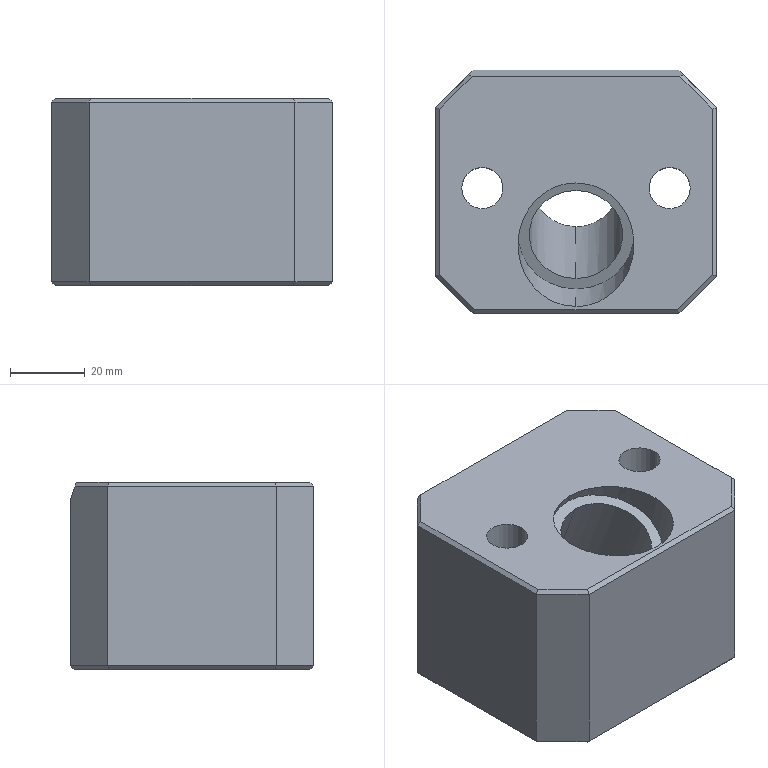Part | Creo | 3 solids | 45 faces | box 75 x 65 x 50 mm | volume 192089 mm3 | plane 29 | cylinder 16 | commonest cylinder face diameters 11 x4 18 x4 11.98 x2 12 x2 25 x2 31 x2
STEP:
#1=CARTESIAN_POINT('',(30.502,321.495,1.));
#2=VERTEX_POINT('',#1);
#3=CARTESIAN_POINT('',(19.502,321.495,1.));
#4=VERTEX_POINT('',#3);
#5=CARTESIAN_POINT('',(25.002,321.495,1.));
#6=DIRECTION('',(0.,0.,1.));
#7=DIRECTION('',(1.,0.,0.));
#8=AXIS2_PLACEMENT_3D('',#5,#6,#7);
#9=CIRCLE('',#8,5.5);
#10=EDGE_CURVE('',#2,#4,#9,.T.);
#11=ORIENTED_EDGE('',*,*,#10,.T.);
#12=CARTESIAN_POINT('',(19.502,321.495,40.));
#13=VERTEX_POINT('',#12);
#14=CARTESIAN_POINT('',(19.502,321.495,1.));
#15=DIRECTION('',(0.,0.,1.));
#16=VECTOR('',#15,39.);
#17=LINE('',#14,#16);
#18=EDGE_CURVE('',#4,#13,#17,.T.);
#19=ORIENTED_EDGE('',*,*,#18,.T.);
#20=CARTESIAN_POINT('',(30.502,321.495,40.));
#21=VERTEX_POINT('',#20);
#22=CARTESIAN_POINT('',(25.002,321.495,40.));
#23=DIRECTION('',(0.,0.,-1.));
#24=DIRECTION('',(-1.,0.,0.));
#25=AXIS2_PLACEMENT_3D('',#22,#23,#24);
#26=CIRCLE('',#25,5.5);
#27=EDGE_CURVE('',#13,#21,#26,.T.);
#28=ORIENTED_EDGE('',*,*,#27,.T.);
#29=CARTESIAN_POINT('',(30.502,321.495,1.));
#30=DIRECTION('',(0.,0.,1.));
#31=VECTOR('',#30,39.);
#32=LINE('',#29,#31);
#33=EDGE_CURVE('',#2,#21,#32,.T.);
#34=ORIENTED_EDGE('',*,*,#33,.F.);
#35=EDGE_LOOP('',(#11,#19,#28,#34));
#36=FACE_OUTER_BOUND('',#35,.F.);
#37=CARTESIAN_POINT('',(25.002,321.495,-10.));
#38=DIRECTION('',(0.,0.,1.));
#39=DIRECTION('',(-1.,0.,0.));
#40=AXIS2_PLACEMENT_3D('',#37,#38,#39);
#41=CYLINDRICAL_SURFACE('',#40,5.5);
#42=ADVANCED_FACE('',(#36),#41,.F.);
#43=CARTESIAN_POINT('',(16.002,321.495,1.));
#44=VERTEX_POINT('',#43);
#45=CARTESIAN_POINT('',(34.002,321.495,1.));
#46=VERTEX_POINT('',#45);
#47=CARTESIAN_POINT('',(25.002,321.495,1.));
#48=DIRECTION('',(0.,0.,-1.));
#49=DIRECTION('',(-1.,0.,0.));
#50=AXIS2_PLACEMENT_3D('',#47,#48,#49);
#51=CIRCLE('',#50,9.);
#52=EDGE_CURVE('',#44,#46,#51,.T.);
#53=ORIENTED_EDGE('',*,*,#52,.F.);
#54=CARTESIAN_POINT('',(25.002,321.495,1.));
#55=DIRECTION('',(0.,0.,-1.));
#56=DIRECTION('',(1.,0.,0.));
#57=AXIS2_PLACEMENT_3D('',#54,#55,#56);
#58=CIRCLE('',#57,9.);
#59=EDGE_CURVE('',#46,#44,#58,.T.);
#60=ORIENTED_EDGE('',*,*,#59,.F.);
#61=EDGE_LOOP('',(#53,#60));
#62=FACE_OUTER_BOUND('',#61,.F.);
#63=CARTESIAN_POINT('',(25.002,321.495,1.));
#64=DIRECTION('',(0.,0.,1.));
#65=DIRECTION('',(-1.,0.,0.));
#66=AXIS2_PLACEMENT_3D('',#63,#64,#65);
#67=CIRCLE('',#66,5.5);
#68=EDGE_CURVE('',#4,#2,#67,.T.);
#69=ORIENTED_EDGE('',*,*,#68,.F.);
#70=ORIENTED_EDGE('',*,*,#10,.F.);
#71=EDGE_LOOP('',(#69,#70));
#72=FACE_BOUND('',#71,.F.);
#73=CARTESIAN_POINT('',(25.002,321.495,1.));
#74=DIRECTION('',(0.,0.,1.));
#75=DIRECTION('',(-1.,0.,0.));
#76=AXIS2_PLACEMENT_3D('',#73,#74,#75);
#77=PLANE('',#76);
#78=ADVANCED_FACE('',(#62,#72),#77,.F.);
#79=ORIENTED_EDGE('',*,*,#52,.T.);
#80=CARTESIAN_POINT('',(34.002,321.495,-10.));
#81=VERTEX_POINT('',#80);
#82=CARTESIAN_POINT('',(34.002,321.495,-10.));
#83=DIRECTION('',(0.,0.,1.));
#84=VECTOR('',#83,11.);
#85=LINE('',#82,#84);
#86=EDGE_CURVE('',#81,#46,#85,.T.);
#87=ORIENTED_EDGE('',*,*,#86,.F.);
#88=CARTESIAN_POINT('',(16.002,321.495,-10.));
#89=VERTEX_POINT('',#88);
#90=CARTESIAN_POINT('',(25.002,321.495,-10.));
#91=DIRECTION('',(0.,0.,1.));
#92=DIRECTION('',(1.,0.,0.));
#93=AXIS2_PLACEMENT_3D('',#90,#91,#92);
#94=CIRCLE('',#93,9.);
#95=EDGE_CURVE('',#81,#89,#94,.T.);
#96=ORIENTED_EDGE('',*,*,#95,.T.);
#97=CARTESIAN_POINT('',(16.002,321.495,-10.));
#98=DIRECTION('',(0.,0.,1.));
#99=VECTOR('',#98,11.);
#100=LINE('',#97,#99);
#101=EDGE_CURVE('',#89,#44,#100,.T.);
#102=ORIENTED_EDGE('',*,*,#101,.T.);
#103=EDGE_LOOP('',(#79,#87,#96,#102));
#104=FACE_OUTER_BOUND('',#103,.F.);
#105=CARTESIAN_POINT('',(25.002,321.495,-10.));
#106=DIRECTION('',(0.,0.,1.));
#107=DIRECTION('',(-1.,0.,0.));
#108=AXIS2_PLACEMENT_3D('',#105,#106,#107);
#109=CYLINDRICAL_SURFACE('',#108,9.);
#110=ADVANCED_FACE('',(#104),#109,.F.);
#111=ORIENTED_EDGE('',*,*,#59,.T.);
#112=ORIENTED_EDGE('',*,*,#101,.F.);
#113=CARTESIAN_POINT('',(25.002,321.495,-10.));
#114=DIRECTION('',(0.,0.,1.));
#115=DIRECTION('',(-1.,0.,0.));
#116=AXIS2_PLACEMENT_3D('',#113,#114,#115);
#117=CIRCLE('',#116,9.);
#118=EDGE_CURVE('',#89,#81,#117,.T.);
#119=ORIENTED_EDGE('',*,*,#118,.T.);
#120=ORIENTED_EDGE('',*,*,#86,.T.);
#121=EDGE_LOOP('',(#111,#112,#119,#120));
#122=FACE_OUTER_BOUND('',#121,.F.);
#123=CARTESIAN_POINT('',(25.002,321.495,-10.));
#124=DIRECTION('',(0.,0.,1.));
#125=DIRECTION('',(-1.,0.,0.));
#126=AXIS2_PLACEMENT_3D('',#123,#124,#125);
#127=CYLINDRICAL_SURFACE('',#126,9.);
#128=ADVANCED_FACE('',(#122),#127,.F.);
#129=CARTESIAN_POINT('',(36.502,298.41,-10.));
#130=VERTEX_POINT('',#129);
#131=CARTESIAN_POINT('',(27.087,288.995,-10.));
#132=VERTEX_POINT('',#131);
#133=CARTESIAN_POINT('',(36.502,298.41,-10.));
#134=DIRECTION('',(-0.7071,-0.7071,0.));
#135=VECTOR('',#134,13.314);
#136=LINE('',#133,#135);
#137=EDGE_CURVE('',#130,#132,#136,.T.);
#138=ORIENTED_EDGE('',*,*,#137,.F.);
#139=CARTESIAN_POINT('',(36.502,342.581,-10.));
#140=VERTEX_POINT('',#139);
#141=CARTESIAN_POINT('',(36.502,298.41,-10.));
#142=DIRECTION('',(0.,1.,0.));
#143=VECTOR('',#142,44.172);
#144=LINE('',#141,#143);
#145=EDGE_CURVE('',#130,#140,#144,.T.);
#146=ORIENTED_EDGE('',*,*,#145,.T.);
#147=CARTESIAN_POINT('',(27.087,351.995,-10.));
#148=VERTEX_POINT('',#147);
#149=CARTESIAN_POINT('',(27.087,351.995,-10.));
#150=DIRECTION('',(0.7071,-0.7071,0.));
#151=VECTOR('',#150,13.314);
#152=LINE('',#149,#151);
#153=EDGE_CURVE('',#148,#140,#152,.T.);
#154=ORIENTED_EDGE('',*,*,#153,.F.);
#155=CARTESIAN_POINT('',(-27.084,351.995,-10.));
#156=VERTEX_POINT('',#155);
#157=CARTESIAN_POINT('',(27.087,351.995,-10.));
#158=DIRECTION('',(-1.,0.,0.));
#159=VECTOR('',#158,54.172);
#160=LINE('',#157,#159);
#161=EDGE_CURVE('',#148,#156,#160,.T.);
#162=ORIENTED_EDGE('',*,*,#161,.T.);
#163=CARTESIAN_POINT('',(-36.498,342.581,-10.));
#164=VERTEX_POINT('',#163);
#165=CARTESIAN_POINT('',(-36.498,342.581,-10.));
#166=DIRECTION('',(0.7071,0.7071,0.));
#167=VECTOR('',#166,13.314);
#168=LINE('',#165,#167);
#169=EDGE_CURVE('',#164,#156,#168,.T.);
#170=ORIENTED_EDGE('',*,*,#169,.F.);
#171=CARTESIAN_POINT('',(-36.498,298.41,-10.));
#172=VERTEX_POINT('',#171);
#173=CARTESIAN_POINT('',(-36.498,342.581,-10.));
#174=DIRECTION('',(0.,-1.,0.));
#175=VECTOR('',#174,44.172);
#176=LINE('',#173,#175);
#177=EDGE_CURVE('',#164,#172,#176,.T.);
#178=ORIENTED_EDGE('',*,*,#177,.T.);
#179=CARTESIAN_POINT('',(-27.084,288.995,-10.));
#180=VERTEX_POINT('',#179);
#181=CARTESIAN_POINT('',(-27.084,288.995,-10.));
#182=DIRECTION('',(-0.7071,0.7071,0.));
#183=VECTOR('',#182,13.314);
#184=LINE('',#181,#183);
#185=EDGE_CURVE('',#180,#172,#184,.T.);
#186=ORIENTED_EDGE('',*,*,#185,.F.);
#187=CARTESIAN_POINT('',(-27.084,288.995,-10.));
#188=DIRECTION('',(1.,0.,0.));
#189=VECTOR('',#188,54.172);
#190=LINE('',#187,#189);
#191=EDGE_CURVE('',#180,#132,#190,.T.);
#192=ORIENTED_EDGE('',*,*,#191,.T.);
#193=EDGE_LOOP('',(#138,#146,#154,#162,#170,#178,#186,#192));
#194=FACE_OUTER_BOUND('',#193,.F.);
#195=ORIENTED_EDGE('',*,*,#118,.F.);
#196=ORIENTED_EDGE('',*,*,#95,.F.);
#197=EDGE_LOOP('',(#195,#196));
#198=FACE_BOUND('',#197,.F.);
#199=CARTESIAN_POINT('',(-33.998,321.495,-10.));
#200=VERTEX_POINT('',#199);
#201=CARTESIAN_POINT('',(-15.998,321.495,-10.));
#202=VERTEX_POINT('',#201);
#203=CARTESIAN_POINT('',(-24.998,321.495,-10.));
#204=DIRECTION('',(0.,0.,1.));
#205=DIRECTION('',(-1.,0.,0.));
#206=AXIS2_PLACEMENT_3D('',#203,#204,#205);
#207=CIRCLE('',#206,9.);
#208=EDGE_CURVE('',#200,#202,#207,.T.);
#209=ORIENTED_EDGE('',*,*,#208,.F.);
#210=CARTESIAN_POINT('',(-24.998,321.495,-10.));
#211=DIRECTION('',(0.,0.,1.));
#212=DIRECTION('',(1.,0.,0.));
#213=AXIS2_PLACEMENT_3D('',#210,#211,#212);
#214=CIRCLE('',#213,9.);
#215=EDGE_CURVE('',#202,#200,#214,.T.);
#216=ORIENTED_EDGE('',*,*,#215,.F.);
#217=EDGE_LOOP('',(#209,#216));
#218=FACE_BOUND('',#217,.F.);
#219=CARTESIAN_POINT('',(0.,311.266,-10.));
#220=VERTEX_POINT('',#219);
#221=CARTESIAN_POINT('',(0.,337.871,-10.));
#222=VERTEX_POINT('',#221);
#223=CARTESIAN_POINT('',(0.,311.266,-10.));
#224=CARTESIAN_POINT('',(-1.473,311.266,-10.));
#225=CARTESIAN_POINT('',(-4.657,311.834,-10.));
#226=CARTESIAN_POINT('',(-8.358,314.374,-10.));
#227=CARTESIAN_POINT('',(-10.541,317.247,-10.));
#228=CARTESIAN_POINT('',(-11.706,319.657,-10.));
#229=CARTESIAN_POINT('',(-12.259,321.74,-10.));
#230=CARTESIAN_POINT('',(-12.467,323.38,-10.));
#231=CARTESIAN_POINT('',(-12.516,324.569,-10.));
#232=CARTESIAN_POINT('',(-12.467,325.757,-10.));
#233=CARTESIAN_POINT('',(-12.259,327.397,-10.));
#234=CARTESIAN_POINT('',(-11.706,329.48,-10.));
#235=CARTESIAN_POINT('',(-10.541,331.89,-10.));
#236=CARTESIAN_POINT('',(-8.358,334.763,-10.));
#237=CARTESIAN_POINT('',(-4.657,337.303,-10.));
#238=CARTESIAN_POINT('',(-1.473,337.871,-10.));
#239=CARTESIAN_POINT('',(0.,337.871,-10.));
#240=B_SPLINE_CURVE_WITH_KNOTS('',3,(#223,#224,#225,#226,#227,#228,#229,#230,#231,#232,#233,#234,#235,#236,#237,#238,#239),.UNSPECIFIED.,.F.,.F.,(4,1,1,1,1,1,1,1,1,1,1,1,1,1,4),(0.,0.125,0.25,0.3125,0.375,0.4375,0.4688,0.5,0.5312,0.5625,0.625,0.6875,0.75,0.875,1.),.UNSPECIFIED.);
#241=EDGE_CURVE('',#220,#222,#240,.T.);
#242=ORIENTED_EDGE('',*,*,#241,.T.);
#243=CARTESIAN_POINT('',(0.,337.871,-10.));
#244=CARTESIAN_POINT('',(1.473,337.871,-10.));
#245=CARTESIAN_POINT('',(4.657,337.303,-10.));
#246=CARTESIAN_POINT('',(8.358,334.763,-10.));
#247=CARTESIAN_POINT('',(10.541,331.89,-10.));
#248=CARTESIAN_POINT('',(11.706,329.48,-10.));
#249=CARTESIAN_POINT('',(12.259,327.397,-10.));
#250=CARTESIAN_POINT('',(12.467,325.757,-10.));
#251=CARTESIAN_POINT('',(12.516,324.569,-10.));
#252=CARTESIAN_POINT('',(12.467,323.38,-10.));
#253=CARTESIAN_POINT('',(12.259,321.74,-10.));
#254=CARTESIAN_POINT('',(11.706,319.657,-10.));
#255=CARTESIAN_POINT('',(10.541,317.247,-10.));
#256=CARTESIAN_POINT('',(8.358,314.374,-10.));
#257=CARTESIAN_POINT('',(4.657,311.834,-10.));
#258=CARTESIAN_POINT('',(1.473,311.266,-10.));
#259=CARTESIAN_POINT('',(0.,311.266,-10.));
#260=B_SPLINE_CURVE_WITH_KNOTS('',3,(#243,#244,#245,#246,#247,#248,#249,#250,#251,#252,#253,#254,#255,#256,#257,#258,#259),.UNSPECIFIED.,.F.,.F.,(4,1,1,1,1,1,1,1,1,1,1,1,1,1,4),(0.,0.125,0.25,0.3125,0.375,0.4375,0.4688,0.5,0.5312,0.5625,0.625,0.6875,0.75,0.875,1.),.UNSPECIFIED.);
#261=EDGE_CURVE('',#222,#220,#260,.T.);
#262=ORIENTED_EDGE('',*,*,#261,.T.);
#263=EDGE_LOOP('',(#242,#262));
#264=FACE_BOUND('',#263,.F.);
#265=CARTESIAN_POINT('',(31.002,-521.005,-10.));
#266=DIRECTION('',(0.,0.,1.));
#267=DIRECTION('',(0.,1.,0.));
#268=AXIS2_PLACEMENT_3D('',#265,#266,#267);
#269=PLANE('',#268);
#270=ADVANCED_FACE('',(#194,#198,#218,#264),#269,.F.);
#271=CARTESIAN_POINT('',(0.,297.353,28.226));
#272=VERTEX_POINT('',#271);
#273=CARTESIAN_POINT('',(0.,320.846,36.776));
#274=VERTEX_POINT('',#273);
#275=CARTESIAN_POINT('',(0.,309.1,32.501));
#276=DIRECTION('',(0.,0.342,-0.9397));
#277=DIRECTION('',(0.,-0.9397,-0.342));
#278=AXIS2_PLACEMENT_3D('',#275,#276,#277);
#279=CIRCLE('',#278,12.5);
#280=EDGE_CURVE('',#272,#274,#279,.T.);
#281=ORIENTED_EDGE('',*,*,#280,.T.);
#282=CARTESIAN_POINT('',(0.,320.846,36.776));
#283=DIRECTION('',(0.,0.342,-0.9397));
#284=VECTOR('',#283,49.778);
#285=LINE('',#282,#284);
#286=EDGE_CURVE('',#274,#222,#285,.T.);
#287=ORIENTED_EDGE('',*,*,#286,.T.);
#288=ORIENTED_EDGE('',*,*,#241,.F.);
#289=CARTESIAN_POINT('',(0.,297.353,28.226));
#290=DIRECTION('',(0.,0.342,-0.9397));
#291=VECTOR('',#290,40.679);
#292=LINE('',#289,#291);
#293=EDGE_CURVE('',#272,#220,#292,.T.);
#294=ORIENTED_EDGE('',*,*,#293,.F.);
#295=EDGE_LOOP('',(#281,#287,#288,#294));
#296=FACE_OUTER_BOUND('',#295,.F.);
#297=CARTESIAN_POINT('',(0.,286.509,94.568));
#298=DIRECTION('',(0.,0.342,-0.9397));
#299=DIRECTION('',(0.,0.9397,0.342));
#300=AXIS2_PLACEMENT_3D('',#297,#298,#299);
#301=CYLINDRICAL_SURFACE('',#300,12.5);
#302=ADVANCED_FACE('',(#296),#301,.F.);
#303=CARTESIAN_POINT('',(0.,294.534,27.2));
#304=VERTEX_POINT('',#303);
#305=CARTESIAN_POINT('',(0.,323.665,37.802));
#306=VERTEX_POINT('',#305);
#307=CARTESIAN_POINT('',(0.,309.1,32.501));
#308=DIRECTION('',(0.,-0.342,0.9397));
#309=DIRECTION('',(0.,-0.9397,-0.342));
#310=AXIS2_PLACEMENT_3D('',#307,#308,#309);
#311=CIRCLE('',#310,15.5);
#312=EDGE_CURVE('',#304,#306,#311,.T.);
#313=ORIENTED_EDGE('',*,*,#312,.F.);
#314=CARTESIAN_POINT('',(0.,309.1,32.501));
#315=DIRECTION('',(0.,-0.342,0.9397));
#316=DIRECTION('',(0.,0.9397,0.342));
#317=AXIS2_PLACEMENT_3D('',#314,#315,#316);
#318=CIRCLE('',#317,15.5);
#319=EDGE_CURVE('',#306,#304,#318,.T.);
#320=ORIENTED_EDGE('',*,*,#319,.F.);
#321=EDGE_LOOP('',(#313,#320));
#322=FACE_OUTER_BOUND('',#321,.F.);
#323=ORIENTED_EDGE('',*,*,#280,.F.);
#324=CARTESIAN_POINT('',(0.,309.1,32.501));
#325=DIRECTION('',(0.,0.342,-0.9397));
#326=DIRECTION('',(0.,0.9397,0.342));
#327=AXIS2_PLACEMENT_3D('',#324,#325,#326);
#328=CIRCLE('',#327,12.5);
#329=EDGE_CURVE('',#274,#272,#328,.T.);
#330=ORIENTED_EDGE('',*,*,#329,.F.);
#331=EDGE_LOOP('',(#323,#330));
#332=FACE_BOUND('',#331,.F.);
#333=CARTESIAN_POINT('',(0.,309.1,32.501));
#334=DIRECTION('',(0.,0.342,-0.9397));
#335=DIRECTION('',(0.,0.9397,0.342));
#336=AXIS2_PLACEMENT_3D('',#333,#334,#335);
#337=PLANE('',#336);
#338=ADVANCED_FACE('',(#322,#332),#337,.F.);
#339=ORIENTED_EDGE('',*,*,#329,.T.);
#340=ORIENTED_EDGE('',*,*,#293,.T.);
#341=ORIENTED_EDGE('',*,*,#261,.F.);
#342=ORIENTED_EDGE('',*,*,#286,.F.);
#343=EDGE_LOOP('',(#339,#340,#341,#342));
#344=FACE_OUTER_BOUND('',#343,.F.);
#345=CARTESIAN_POINT('',(0.,286.509,94.568));
#346=DIRECTION('',(0.,0.342,-0.9397));
#347=DIRECTION('',(0.,0.9397,0.342));
#348=AXIS2_PLACEMENT_3D('',#345,#346,#347);
#349=CYLINDRICAL_SURFACE('',#348,12.5);
#350=ADVANCED_FACE('',(#344),#349,.F.);
#351=CARTESIAN_POINT('',(0.,322.865,40.));
#352=VERTEX_POINT('',#351);
#353=CARTESIAN_POINT('',(0.,289.875,40.));
#354=VERTEX_POINT('',#353);
#355=CARTESIAN_POINT('',(0.,322.865,40.));
#356=CARTESIAN_POINT('',(1.827,322.865,40.));
#357=CARTESIAN_POINT('',(5.775,322.161,40.));
#358=CARTESIAN_POINT('',(10.364,319.011,40.));
#359=CARTESIAN_POINT('',(13.071,315.449,40.));
#360=CARTESIAN_POINT('',(14.515,312.46,40.));
#361=CARTESIAN_POINT('',(15.201,309.877,40.));
#362=CARTESIAN_POINT('',(15.46,307.844,40.));
#363=CARTESIAN_POINT('',(15.52,306.37,40.));
#364=CARTESIAN_POINT('',(15.46,304.897,40.));
#365=CARTESIAN_POINT('',(15.201,302.863,40.));
#366=CARTESIAN_POINT('',(14.515,300.28,40.));
#367=CARTESIAN_POINT('',(13.071,297.291,40.));
#368=CARTESIAN_POINT('',(10.364,293.729,40.));
#369=CARTESIAN_POINT('',(5.775,290.58,40.));
#370=CARTESIAN_POINT('',(1.827,289.875,40.));
#371=CARTESIAN_POINT('',(0.,289.875,40.));
#372=B_SPLINE_CURVE_WITH_KNOTS('',3,(#355,#356,#357,#358,#359,#360,#361,#362,#363,#364,#365,#366,#367,#368,#369,#370,#371),.UNSPECIFIED.,.F.,.F.,(4,1,1,1,1,1,1,1,1,1,1,1,1,1,4),(0.,0.125,0.25,0.3125,0.375,0.4375,0.4688,0.5,0.5312,0.5625,0.625,0.6875,0.75,0.875,1.),.UNSPECIFIED.);
#373=EDGE_CURVE('',#352,#354,#372,.T.);
#374=ORIENTED_EDGE('',*,*,#373,.T.);
#375=CARTESIAN_POINT('',(0.,289.875,40.));
#376=DIRECTION('',(0.,0.342,-0.9397));
#377=VECTOR('',#376,13.622);
#378=LINE('',#375,#377);
#379=EDGE_CURVE('',#354,#304,#378,.T.);
#380=ORIENTED_EDGE('',*,*,#379,.T.);
#381=ORIENTED_EDGE('',*,*,#312,.T.);
#382=CARTESIAN_POINT('',(0.,322.865,40.));
#383=DIRECTION('',(0.,0.342,-0.9397));
#384=VECTOR('',#383,2.339);
#385=LINE('',#382,#384);
#386=EDGE_CURVE('',#352,#306,#385,.T.);
#387=ORIENTED_EDGE('',*,*,#386,.F.);
#388=EDGE_LOOP('',(#374,#380,#381,#387));
#389=FACE_OUTER_BOUND('',#388,.F.);
#390=CARTESIAN_POINT('',(0.,302.516,50.59));
#391=DIRECTION('',(0.,0.342,-0.9397));
#392=DIRECTION('',(0.,0.9397,0.342));
#393=AXIS2_PLACEMENT_3D('',#390,#391,#392);
#394=CYLINDRICAL_SURFACE('',#393,15.5);
#395=ADVANCED_FACE('',(#389),#394,.F.);
#396=CARTESIAN_POINT('',(27.723,351.359,40.));
#397=VERTEX_POINT('',#396);
#398=CARTESIAN_POINT('',(-27.72,351.359,40.));
#399=VERTEX_POINT('',#398);
#400=CARTESIAN_POINT('',(27.723,351.359,40.));
#401=DIRECTION('',(-1.,0.,0.));
#402=VECTOR('',#401,55.444);
#403=LINE('',#400,#402);
#404=EDGE_CURVE('',#397,#399,#403,.T.);
#405=ORIENTED_EDGE('',*,*,#404,.F.);
#406=CARTESIAN_POINT('',(36.502,342.581,40.));
#407=VERTEX_POINT('',#406);
#408=CARTESIAN_POINT('',(36.502,342.581,40.));
#409=DIRECTION('',(-0.7071,0.7071,0.));
#410=VECTOR('',#409,12.414);
#411=LINE('',#408,#410);
#412=EDGE_CURVE('',#407,#397,#411,.T.);
#413=ORIENTED_EDGE('',*,*,#412,.F.);
#414=CARTESIAN_POINT('',(36.502,298.41,40.));
#415=VERTEX_POINT('',#414);
#416=CARTESIAN_POINT('',(36.502,342.581,40.));
#417=DIRECTION('',(0.,-1.,0.));
#418=VECTOR('',#417,44.172);
#419=LINE('',#416,#418);
#420=EDGE_CURVE('',#407,#415,#419,.T.);
#421=ORIENTED_EDGE('',*,*,#420,.T.);
#422=CARTESIAN_POINT('',(27.087,288.995,40.));
#423=VERTEX_POINT('',#422);
#424=CARTESIAN_POINT('',(27.087,288.995,40.));
#425=DIRECTION('',(0.7071,0.7071,0.));
#426=VECTOR('',#425,13.314);
#427=LINE('',#424,#426);
#428=EDGE_CURVE('',#423,#415,#427,.T.);
#429=ORIENTED_EDGE('',*,*,#428,.F.);
#430=CARTESIAN_POINT('',(-27.084,288.995,40.));
#431=VERTEX_POINT('',#430);
#432=CARTESIAN_POINT('',(27.087,288.995,40.));
#433=DIRECTION('',(-1.,0.,0.));
#434=VECTOR('',#433,54.172);
#435=LINE('',#432,#434);
#436=EDGE_CURVE('',#423,#431,#435,.T.);
#437=ORIENTED_EDGE('',*,*,#436,.T.);
#438=CARTESIAN_POINT('',(-36.498,298.41,40.));
#439=VERTEX_POINT('',#438);
#440=CARTESIAN_POINT('',(-36.498,298.41,40.));
#441=DIRECTION('',(0.7071,-0.7071,0.));
#442=VECTOR('',#441,13.314);
#443=LINE('',#440,#442);
#444=EDGE_CURVE('',#439,#431,#443,.T.);
#445=ORIENTED_EDGE('',*,*,#444,.F.);
#446=CARTESIAN_POINT('',(-36.498,342.581,40.));
#447=VERTEX_POINT('',#446);
#448=CARTESIAN_POINT('',(-36.498,298.41,40.));
#449=DIRECTION('',(0.,1.,0.));
#450=VECTOR('',#449,44.172);
#451=LINE('',#448,#450);
#452=EDGE_CURVE('',#439,#447,#451,.T.);
#453=ORIENTED_EDGE('',*,*,#452,.T.);
#454=CARTESIAN_POINT('',(-27.72,351.359,40.));
#455=DIRECTION('',(-0.7071,-0.7071,0.));
#456=VECTOR('',#455,12.414);
#457=LINE('',#454,#456);
#458=EDGE_CURVE('',#399,#447,#457,.T.);
#459=ORIENTED_EDGE('',*,*,#458,.F.);
#460=EDGE_LOOP('',(#405,#413,#421,#429,#437,#445,#453,#459));
#461=FACE_OUTER_BOUND('',#460,.F.);
#462=ORIENTED_EDGE('',*,*,#27,.F.);
#463=CARTESIAN_POINT('',(25.002,321.495,40.));
#464=DIRECTION('',(0.,0.,-1.));
#465=DIRECTION('',(1.,0.,0.));
#466=AXIS2_PLACEMENT_3D('',#463,#464,#465);
#467=CIRCLE('',#466,5.5);
#468=EDGE_CURVE('',#21,#13,#467,.T.);
#469=ORIENTED_EDGE('',*,*,#468,.F.);
#470=EDGE_LOOP('',(#462,#469));
#471=FACE_BOUND('',#470,.F.);
#472=CARTESIAN_POINT('',(-30.498,321.495,40.));
#473=VERTEX_POINT('',#472);
#474=CARTESIAN_POINT('',(-19.498,321.495,40.));
#475=VERTEX_POINT('',#474);
#476=CARTESIAN_POINT('',(-24.998,321.495,40.));
#477=DIRECTION('',(0.,0.,-1.));
#478=DIRECTION('',(-1.,0.,0.));
#479=AXIS2_PLACEMENT_3D('',#476,#477,#478);
#480=CIRCLE('',#479,5.5);
#481=EDGE_CURVE('',#473,#475,#480,.T.);
#482=ORIENTED_EDGE('',*,*,#481,.F.);
#483=CARTESIAN_POINT('',(-24.998,321.495,40.));
#484=DIRECTION('',(0.,0.,-1.));
#485=DIRECTION('',(1.,0.,0.));
#486=AXIS2_PLACEMENT_3D('',#483,#484,#485);
#487=CIRCLE('',#486,5.5);
#488=EDGE_CURVE('',#475,#473,#487,.T.);
#489=ORIENTED_EDGE('',*,*,#488,.F.);
#490=EDGE_LOOP('',(#482,#489));
#491=FACE_BOUND('',#490,.F.);
#492=ORIENTED_EDGE('',*,*,#373,.F.);
#493=CARTESIAN_POINT('',(0.,289.875,40.));
#494=CARTESIAN_POINT('',(-1.827,289.875,40.));
#495=CARTESIAN_POINT('',(-5.775,290.58,40.));
#496=CARTESIAN_POINT('',(-10.364,293.729,40.));
#497=CARTESIAN_POINT('',(-13.071,297.291,40.));
#498=CARTESIAN_POINT('',(-14.515,300.28,40.));
#499=CARTESIAN_POINT('',(-15.201,302.863,40.));
#500=CARTESIAN_POINT('',(-15.46,304.897,40.));
#501=CARTESIAN_POINT('',(-15.52,306.37,40.));
#502=CARTESIAN_POINT('',(-15.46,307.844,40.));
#503=CARTESIAN_POINT('',(-15.201,309.877,40.));
#504=CARTESIAN_POINT('',(-14.515,312.46,40.));
#505=CARTESIAN_POINT('',(-13.071,315.449,40.));
#506=CARTESIAN_POINT('',(-10.364,319.011,40.));
#507=CARTESIAN_POINT('',(-5.775,322.161,40.));
#508=CARTESIAN_POINT('',(-1.827,322.865,40.));
#509=CARTESIAN_POINT('',(0.,322.865,40.));
#510=B_SPLINE_CURVE_WITH_KNOTS('',3,(#493,#494,#495,#496,#497,#498,#499,#500,#501,#502,#503,#504,#505,#506,#507,#508,#509),.UNSPECIFIED.,.F.,.F.,(4,1,1,1,1,1,1,1,1,1,1,1,1,1,4),(0.,0.125,0.25,0.3125,0.375,0.4375,0.4688,0.5,0.5312,0.5625,0.625,0.6875,0.75,0.875,1.),.UNSPECIFIED.);
#511=EDGE_CURVE('',#354,#352,#510,.T.);
#512=ORIENTED_EDGE('',*,*,#511,.F.);
#513=EDGE_LOOP('',(#492,#512));
#514=FACE_BOUND('',#513,.F.);
#515=CARTESIAN_POINT('',(-365.934,307.393,40.));
#516=DIRECTION('',(0.,0.,1.));
#517=DIRECTION('',(1.,0.,0.));
#518=AXIS2_PLACEMENT_3D('',#515,#516,#517);
#519=PLANE('',#518);
#520=ADVANCED_FACE('',(#461,#471,#491,#514),#519,.T.);
#521=CARTESIAN_POINT('',(-28.771,351.723,39.));
#522=VERTEX_POINT('',#521);
#523=CARTESIAN_POINT('',(-27.498,352.995,35.505));
#524=VERTEX_POINT('',#523);
#525=CARTESIAN_POINT('',(-28.771,351.723,39.));
#526=DIRECTION('',(0.3236,0.3236,-0.8891));
#527=VECTOR('',#526,3.931);
#528=LINE('',#525,#527);
#529=EDGE_CURVE('',#522,#524,#528,.T.);
#530=ORIENTED_EDGE('',*,*,#529,.T.);
#531=CARTESIAN_POINT('',(27.502,352.995,35.505));
#532=VERTEX_POINT('',#531);
#533=CARTESIAN_POINT('',(-27.498,352.995,35.505));
#534=DIRECTION('',(1.,0.,0.));
#535=VECTOR('',#534,55.);
#536=LINE('',#533,#535);
#537=EDGE_CURVE('',#524,#532,#536,.T.);
#538=ORIENTED_EDGE('',*,*,#537,.T.);
#539=CARTESIAN_POINT('',(28.774,351.723,39.));
#540=VERTEX_POINT('',#539);
#541=CARTESIAN_POINT('',(28.774,351.723,39.));
#542=DIRECTION('',(-0.3236,0.3236,-0.8891));
#543=VECTOR('',#542,3.931);
#544=LINE('',#541,#543);
#545=EDGE_CURVE('',#540,#532,#544,.T.);
#546=ORIENTED_EDGE('',*,*,#545,.F.);
#547=CARTESIAN_POINT('',(28.774,351.723,39.));
#548=DIRECTION('',(-0.7024,-0.2434,0.6688));
#549=VECTOR('',#548,1.495);
#550=LINE('',#547,#549);
#551=EDGE_CURVE('',#540,#397,#550,.T.);
#552=ORIENTED_EDGE('',*,*,#551,.T.);
#553=ORIENTED_EDGE('',*,*,#404,.T.);
#554=CARTESIAN_POINT('',(-28.771,351.723,39.));
#555=DIRECTION('',(0.7024,-0.2434,0.6688));
#556=VECTOR('',#555,1.495);
#557=LINE('',#554,#556);
#558=EDGE_CURVE('',#522,#399,#557,.T.);
#559=ORIENTED_EDGE('',*,*,#558,.F.);
#560=EDGE_LOOP('',(#530,#538,#546,#552,#553,#559));
#561=FACE_OUTER_BOUND('',#560,.F.);
#562=CARTESIAN_POINT('',(0.00154,350.995,41.));
#563=DIRECTION('',(0.,0.9397,0.342));
#564=DIRECTION('',(0.,-0.342,0.9397));
#565=AXIS2_PLACEMENT_3D('',#562,#563,#564);
#566=PLANE('',#565);
#567=ADVANCED_FACE('',(#561),#566,.T.);
#568=ORIENTED_EDGE('',*,*,#529,.F.);
#569=CARTESIAN_POINT('',(-37.498,342.995,39.));
#570=VERTEX_POINT('',#569);
#571=CARTESIAN_POINT('',(-28.771,351.723,39.));
#572=DIRECTION('',(-0.7071,-0.7071,0.));
#573=VECTOR('',#572,12.343);
#574=LINE('',#571,#573);
#575=EDGE_CURVE('',#522,#570,#574,.T.);
#576=ORIENTED_EDGE('',*,*,#575,.T.);
#577=CARTESIAN_POINT('',(-37.498,342.995,-9.));
#578=VERTEX_POINT('',#577);
#579=CARTESIAN_POINT('',(-37.498,342.995,-9.));
#580=DIRECTION('',(0.,0.,1.));
#581=VECTOR('',#580,48.);
#582=LINE('',#579,#581);
#583=EDGE_CURVE('',#578,#570,#582,.T.);
#584=ORIENTED_EDGE('',*,*,#583,.F.);
#585=CARTESIAN_POINT('',(-27.498,352.995,-9.));
#586=VERTEX_POINT('',#585);
#587=CARTESIAN_POINT('',(-37.498,342.995,-9.));
#588=DIRECTION('',(0.7071,0.7071,0.));
#589=VECTOR('',#588,14.142);
#590=LINE('',#587,#589);
#591=EDGE_CURVE('',#578,#586,#590,.T.);
#592=ORIENTED_EDGE('',*,*,#591,.T.);
#593=CARTESIAN_POINT('',(-27.498,352.995,35.505));
#594=DIRECTION('',(0.,0.,-1.));
#595=VECTOR('',#594,44.505);
#596=LINE('',#593,#595);
#597=EDGE_CURVE('',#524,#586,#596,.T.);
#598=ORIENTED_EDGE('',*,*,#597,.F.);
#599=EDGE_LOOP('',(#568,#576,#584,#592,#598));
#600=FACE_OUTER_BOUND('',#599,.F.);
#601=CARTESIAN_POINT('',(-37.498,342.995,-66.89));
#602=DIRECTION('',(-0.7071,0.7071,0.));
#603=DIRECTION('',(0.,0.,1.));
#604=AXIS2_PLACEMENT_3D('',#601,#602,#603);
#605=PLANE('',#604);
#606=ADVANCED_FACE('',(#600),#605,.T.);
#607=ORIENTED_EDGE('',*,*,#458,.T.);
#608=CARTESIAN_POINT('',(-37.498,342.995,39.));
#609=DIRECTION('',(0.6786,-0.2811,0.6786));
#610=VECTOR('',#609,1.474);
#611=LINE('',#608,#610);
#612=EDGE_CURVE('',#570,#447,#611,.T.);
#613=ORIENTED_EDGE('',*,*,#612,.F.);
#614=ORIENTED_EDGE('',*,*,#575,.F.);
#615=ORIENTED_EDGE('',*,*,#558,.T.);
#616=EDGE_LOOP('',(#607,#613,#614,#615));
#617=FACE_OUTER_BOUND('',#616,.F.);
#618=CARTESIAN_POINT('',(-218.811,160.269,40.));
#619=DIRECTION('',(0.5,-0.5,-0.7071));
#620=DIRECTION('',(-0.7071,-0.7071,0.));
#621=AXIS2_PLACEMENT_3D('',#618,#619,#620);
#622=PLANE('',#621);
#623=ADVANCED_FACE('',(#617),#622,.F.);
#624=ORIENTED_EDGE('',*,*,#612,.T.);
#625=ORIENTED_EDGE('',*,*,#452,.F.);
#626=CARTESIAN_POINT('',(-37.498,297.995,39.));
#627=VERTEX_POINT('',#626);
#628=CARTESIAN_POINT('',(-37.498,297.995,39.));
#629=DIRECTION('',(0.6786,0.2811,0.6786));
#630=VECTOR('',#629,1.474);
#631=LINE('',#628,#630);
#632=EDGE_CURVE('',#627,#439,#631,.T.);
#633=ORIENTED_EDGE('',*,*,#632,.F.);
#634=CARTESIAN_POINT('',(-37.498,342.995,39.));
#635=DIRECTION('',(0.,-1.,0.));
#636=VECTOR('',#635,45.);
#637=LINE('',#634,#636);
#638=EDGE_CURVE('',#570,#627,#637,.T.);
#639=ORIENTED_EDGE('',*,*,#638,.F.);
#640=EDGE_LOOP('',(#624,#625,#633,#639));
#641=FACE_OUTER_BOUND('',#640,.F.);
#642=CARTESIAN_POINT('',(-36.498,307.393,40.));
#643=DIRECTION('',(-0.7071,0.,0.7071));
#644=DIRECTION('',(0.,1.,0.));
#645=AXIS2_PLACEMENT_3D('',#642,#643,#644);
#646=PLANE('',#645);
#647=ADVANCED_FACE('',(#641),#646,.T.);
#648=ORIENTED_EDGE('',*,*,#632,.T.);
#649=ORIENTED_EDGE('',*,*,#444,.T.);
#650=CARTESIAN_POINT('',(-27.498,287.995,39.));
#651=VERTEX_POINT('',#650);
#652=CARTESIAN_POINT('',(-27.498,287.995,39.));
#653=DIRECTION('',(0.2811,0.6786,0.6786));
#654=VECTOR('',#653,1.474);
#655=LINE('',#652,#654);
#656=EDGE_CURVE('',#651,#431,#655,.T.);
#657=ORIENTED_EDGE('',*,*,#656,.F.);
#658=CARTESIAN_POINT('',(-37.498,297.995,39.));
#659=DIRECTION('',(0.7071,-0.7071,0.));
#660=VECTOR('',#659,14.142);
#661=LINE('',#658,#660);
#662=EDGE_CURVE('',#627,#651,#661,.T.);
#663=ORIENTED_EDGE('',*,*,#662,.F.);
#664=EDGE_LOOP('',(#648,#649,#657,#663));
#665=FACE_OUTER_BOUND('',#664,.F.);
#666=CARTESIAN_POINT('',(-205.708,467.619,40.));
#667=DIRECTION('',(0.5,0.5,-0.7071));
#668=DIRECTION('',(0.7071,-0.7071,0.));
#669=AXIS2_PLACEMENT_3D('',#666,#667,#668);
#670=PLANE('',#669);
#671=ADVANCED_FACE('',(#665),#670,.F.);
#672=CARTESIAN_POINT('',(27.502,287.995,39.));
#673=VERTEX_POINT('',#672);
#674=CARTESIAN_POINT('',(27.502,287.995,39.));
#675=DIRECTION('',(-0.2811,0.6786,0.6786));
#676=VECTOR('',#675,1.474);
#677=LINE('',#674,#676);
#678=EDGE_CURVE('',#673,#423,#677,.T.);
#679=ORIENTED_EDGE('',*,*,#678,.F.);
#680=CARTESIAN_POINT('',(-27.498,287.995,39.));
#681=DIRECTION('',(1.,0.,0.));
#682=VECTOR('',#681,55.);
#683=LINE('',#680,#682);
#684=EDGE_CURVE('',#651,#673,#683,.T.);
#685=ORIENTED_EDGE('',*,*,#684,.F.);
#686=ORIENTED_EDGE('',*,*,#656,.T.);
#687=ORIENTED_EDGE('',*,*,#436,.F.);
#688=EDGE_LOOP('',(#679,#685,#686,#687));
#689=FACE_OUTER_BOUND('',#688,.F.);
#690=CARTESIAN_POINT('',(-278.498,287.995,39.));
#691=DIRECTION('',(0.,0.7071,-0.7071));
#692=DIRECTION('',(-1.,0.,0.));
#693=AXIS2_PLACEMENT_3D('',#690,#691,#692);
#694=PLANE('',#693);
#695=ADVANCED_FACE('',(#689),#694,.F.);
#696=ORIENTED_EDGE('',*,*,#678,.T.);
#697=ORIENTED_EDGE('',*,*,#428,.T.);
#698=CARTESIAN_POINT('',(37.502,297.995,39.));
#699=VERTEX_POINT('',#698);
#700=CARTESIAN_POINT('',(36.502,298.41,40.));
#701=DIRECTION('',(0.6786,-0.2811,-0.6786));
#702=VECTOR('',#701,1.474);
#703=LINE('',#700,#702);
#704=EDGE_CURVE('',#415,#699,#703,.T.);
#705=ORIENTED_EDGE('',*,*,#704,.T.);
#706=CARTESIAN_POINT('',(27.502,287.995,39.));
#707=DIRECTION('',(0.7071,0.7071,0.));
#708=VECTOR('',#707,14.142);
#709=LINE('',#706,#708);
#710=EDGE_CURVE('',#673,#699,#709,.T.);
#711=ORIENTED_EDGE('',*,*,#710,.F.);
#712=EDGE_LOOP('',(#696,#697,#705,#711));
#713=FACE_OUTER_BOUND('',#712,.F.);
#714=CARTESIAN_POINT('',(-160.225,101.683,40.));
#715=DIRECTION('',(0.5,-0.5,0.7071));
#716=DIRECTION('',(-0.7071,-0.7071,0.));
#717=AXIS2_PLACEMENT_3D('',#714,#715,#716);
#718=PLANE('',#717);
#719=ADVANCED_FACE('',(#713),#718,.T.);
#720=CARTESIAN_POINT('',(37.502,342.995,39.));
#721=VERTEX_POINT('',#720);
#722=CARTESIAN_POINT('',(36.502,342.581,40.));
#723=DIRECTION('',(0.6786,0.2811,-0.6786));
#724=VECTOR('',#723,1.474);
#725=LINE('',#722,#724);
#726=EDGE_CURVE('',#407,#721,#725,.T.);
#727=ORIENTED_EDGE('',*,*,#726,.T.);
#728=CARTESIAN_POINT('',(37.502,297.995,39.));
#729=DIRECTION('',(0.,1.,0.));
#730=VECTOR('',#729,45.);
#731=LINE('',#728,#730);
#732=EDGE_CURVE('',#699,#721,#731,.T.);
#733=ORIENTED_EDGE('',*,*,#732,.F.);
#734=ORIENTED_EDGE('',*,*,#704,.F.);
#735=ORIENTED_EDGE('',*,*,#420,.F.);
#736=EDGE_LOOP('',(#727,#733,#734,#735));
#737=FACE_OUTER_BOUND('',#736,.F.);
#738=CARTESIAN_POINT('',(36.502,307.393,40.));
#739=DIRECTION('',(-0.7071,0.,-0.7071));
#740=DIRECTION('',(0.,1.,0.));
#741=AXIS2_PLACEMENT_3D('',#738,#739,#740);
#742=PLANE('',#741);
#743=ADVANCED_FACE('',(#737),#742,.F.);
#744=ORIENTED_EDGE('',*,*,#551,.F.);
#745=CARTESIAN_POINT('',(37.502,342.995,39.));
#746=DIRECTION('',(-0.7071,0.7071,0.));
#747=VECTOR('',#746,12.343);
#748=LINE('',#745,#747);
#749=EDGE_CURVE('',#721,#540,#748,.T.);
#750=ORIENTED_EDGE('',*,*,#749,.F.);
#751=ORIENTED_EDGE('',*,*,#726,.F.);
#752=ORIENTED_EDGE('',*,*,#412,.T.);
#753=EDGE_LOOP('',(#744,#750,#751,#752));
#754=FACE_OUTER_BOUND('',#753,.F.);
#755=CARTESIAN_POINT('',(-147.122,526.205,40.));
#756=DIRECTION('',(0.5,0.5,0.7071));
#757=DIRECTION('',(0.7071,-0.7071,0.));
#758=AXIS2_PLACEMENT_3D('',#755,#756,#757);
#759=PLANE('',#758);
#760=ADVANCED_FACE('',(#754),#759,.T.);
#761=CARTESIAN_POINT('',(27.502,352.995,-9.));
#762=VERTEX_POINT('',#761);
#763=CARTESIAN_POINT('',(27.502,352.995,-9.));
#764=DIRECTION('',(0.,0.,1.));
#765=VECTOR('',#764,44.505);
#766=LINE('',#763,#765);
#767=EDGE_CURVE('',#762,#532,#766,.T.);
#768=ORIENTED_EDGE('',*,*,#767,.F.);
#769=CARTESIAN_POINT('',(37.502,342.995,-9.));
#770=VERTEX_POINT('',#769);
#771=CARTESIAN_POINT('',(27.502,352.995,-9.));
#772=DIRECTION('',(0.7071,-0.7071,0.));
#773=VECTOR('',#772,14.142);
#774=LINE('',#771,#773);
#775=EDGE_CURVE('',#762,#770,#774,.T.);
#776=ORIENTED_EDGE('',*,*,#775,.T.);
#777=CARTESIAN_POINT('',(37.502,342.995,39.));
#778=DIRECTION('',(0.,0.,-1.));
#779=VECTOR('',#778,48.);
#780=LINE('',#777,#779);
#781=EDGE_CURVE('',#721,#770,#780,.T.);
#782=ORIENTED_EDGE('',*,*,#781,.F.);
#783=ORIENTED_EDGE('',*,*,#749,.T.);
#784=ORIENTED_EDGE('',*,*,#545,.T.);
#785=EDGE_LOOP('',(#768,#776,#782,#783,#784));
#786=FACE_OUTER_BOUND('',#785,.F.);
#787=CARTESIAN_POINT('',(27.502,352.995,-20.39));
#788=DIRECTION('',(-0.7071,-0.7071,0.));
#789=DIRECTION('',(0.,0.,-1.));
#790=AXIS2_PLACEMENT_3D('',#787,#788,#789);
#791=PLANE('',#790);
#792=ADVANCED_FACE('',(#786),#791,.F.);
#793=ORIENTED_EDGE('',*,*,#537,.F.);
#794=ORIENTED_EDGE('',*,*,#597,.T.);
#795=CARTESIAN_POINT('',(-27.498,352.995,-9.));
#796=DIRECTION('',(1.,0.,0.));
#797=VECTOR('',#796,55.);
#798=LINE('',#795,#797);
#799=EDGE_CURVE('',#586,#762,#798,.T.);
#800=ORIENTED_EDGE('',*,*,#799,.T.);
#801=ORIENTED_EDGE('',*,*,#767,.T.);
#802=EDGE_LOOP('',(#793,#794,#800,#801));
#803=FACE_OUTER_BOUND('',#802,.F.);
#804=CARTESIAN_POINT('',(-189.995,352.995,-20.39));
#805=DIRECTION('',(0.,1.,0.));
#806=DIRECTION('',(0.,0.,-1.));
#807=AXIS2_PLACEMENT_3D('',#804,#805,#806);
#808=PLANE('',#807);
#809=ADVANCED_FACE('',(#803),#808,.T.);
#810=CARTESIAN_POINT('',(27.087,351.995,-10.));
#811=DIRECTION('',(0.2811,0.6786,0.6786));
#812=VECTOR('',#811,1.474);
#813=LINE('',#810,#812);
#814=EDGE_CURVE('',#148,#762,#813,.T.);
#815=ORIENTED_EDGE('',*,*,#814,.T.);
#816=ORIENTED_EDGE('',*,*,#799,.F.);
#817=CARTESIAN_POINT('',(-27.084,351.995,-10.));
#818=DIRECTION('',(-0.2811,0.6786,0.6786));
#819=VECTOR('',#818,1.474);
#820=LINE('',#817,#819);
#821=EDGE_CURVE('',#156,#586,#820,.T.);
#822=ORIENTED_EDGE('',*,*,#821,.F.);
#823=ORIENTED_EDGE('',*,*,#161,.F.);
#824=EDGE_LOOP('',(#815,#816,#822,#823));
#825=FACE_OUTER_BOUND('',#824,.F.);
#826=CARTESIAN_POINT('',(-189.995,352.995,-9.));
#827=DIRECTION('',(0.,0.7071,-0.7071));
#828=DIRECTION('',(1.,0.,0.));
#829=AXIS2_PLACEMENT_3D('',#826,#827,#828);
#830=PLANE('',#829);
#831=ADVANCED_FACE('',(#825),#830,.T.);
#832=CARTESIAN_POINT('',(36.502,342.581,-10.));
#833=DIRECTION('',(0.6786,0.2811,0.6786));
#834=VECTOR('',#833,1.474);
#835=LINE('',#832,#834);
#836=EDGE_CURVE('',#140,#770,#835,.T.);
#837=ORIENTED_EDGE('',*,*,#836,.T.);
#838=ORIENTED_EDGE('',*,*,#775,.F.);
#839=ORIENTED_EDGE('',*,*,#814,.F.);
#840=ORIENTED_EDGE('',*,*,#153,.T.);
#841=EDGE_LOOP('',(#837,#838,#839,#840));
#842=FACE_OUTER_BOUND('',#841,.F.);
#843=CARTESIAN_POINT('',(465.544,-86.462,-10.));
#844=DIRECTION('',(-0.5,-0.5,0.7071));
#845=DIRECTION('',(0.7071,-0.7071,0.));
#846=AXIS2_PLACEMENT_3D('',#843,#844,#845);
#847=PLANE('',#846);
#848=ADVANCED_FACE('',(#842),#847,.F.);
#849=CARTESIAN_POINT('',(37.502,297.995,-9.));
#850=VERTEX_POINT('',#849);
#851=CARTESIAN_POINT('',(37.502,342.995,-9.));
#852=DIRECTION('',(0.,-1.,0.));
#853=VECTOR('',#852,45.);
#854=LINE('',#851,#853);
#855=EDGE_CURVE('',#770,#850,#854,.T.);
#856=ORIENTED_EDGE('',*,*,#855,.F.);
#857=ORIENTED_EDGE('',*,*,#836,.F.);
#858=ORIENTED_EDGE('',*,*,#145,.F.);
#859=CARTESIAN_POINT('',(36.502,298.41,-10.));
#860=DIRECTION('',(0.6786,-0.2811,0.6786));
#861=VECTOR('',#860,1.474);
#862=LINE('',#859,#861);
#863=EDGE_CURVE('',#130,#850,#862,.T.);
#864=ORIENTED_EDGE('',*,*,#863,.T.);
#865=EDGE_LOOP('',(#856,#857,#858,#864));
#866=FACE_OUTER_BOUND('',#865,.F.);
#867=CARTESIAN_POINT('',(36.502,-521.005,-10.));
#868=DIRECTION('',(0.7071,0.,-0.7071));
#869=DIRECTION('',(0.,1.,0.));
#870=AXIS2_PLACEMENT_3D('',#867,#868,#869);
#871=PLANE('',#870);
#872=ADVANCED_FACE('',(#866),#871,.T.);
#873=CARTESIAN_POINT('',(37.502,297.995,-9.));
#874=DIRECTION('',(0.,0.,1.));
#875=VECTOR('',#874,48.);
#876=LINE('',#873,#875);
#877=EDGE_CURVE('',#850,#699,#876,.T.);
#878=ORIENTED_EDGE('',*,*,#877,.T.);
#879=ORIENTED_EDGE('',*,*,#732,.T.);
#880=ORIENTED_EDGE('',*,*,#781,.T.);
#881=ORIENTED_EDGE('',*,*,#855,.T.);
#882=EDGE_LOOP('',(#878,#879,#880,#881));
#883=FACE_OUTER_BOUND('',#882,.F.);
#884=CARTESIAN_POINT('',(37.502,292.393,49.24));
#885=DIRECTION('',(1.,0.,0.));
#886=DIRECTION('',(0.,0.,-1.));
#887=AXIS2_PLACEMENT_3D('',#884,#885,#886);
#888=PLANE('',#887);
#889=ADVANCED_FACE('',(#883),#888,.T.);
#890=CARTESIAN_POINT('',(27.502,287.995,-9.));
#891=VERTEX_POINT('',#890);
#892=CARTESIAN_POINT('',(27.502,287.995,39.));
#893=DIRECTION('',(0.,0.,-1.));
#894=VECTOR('',#893,48.);
#895=LINE('',#892,#894);
#896=EDGE_CURVE('',#673,#891,#895,.T.);
#897=ORIENTED_EDGE('',*,*,#896,.F.);
#898=ORIENTED_EDGE('',*,*,#710,.T.);
#899=ORIENTED_EDGE('',*,*,#877,.F.);
#900=CARTESIAN_POINT('',(37.502,297.995,-9.));
#901=DIRECTION('',(-0.7071,-0.7071,0.));
#902=VECTOR('',#901,14.142);
#903=LINE('',#900,#902);
#904=EDGE_CURVE('',#850,#891,#903,.T.);
#905=ORIENTED_EDGE('',*,*,#904,.T.);
#906=EDGE_LOOP('',(#897,#898,#899,#905));
#907=FACE_OUTER_BOUND('',#906,.F.);
#908=CARTESIAN_POINT('',(27.502,287.995,19.62));
#909=DIRECTION('',(-0.7071,0.7071,0.));
#910=DIRECTION('',(0.,0.,1.));
#911=AXIS2_PLACEMENT_3D('',#908,#909,#910);
#912=PLANE('',#911);
#913=ADVANCED_FACE('',(#907),#912,.F.);
#914=CARTESIAN_POINT('',(-27.498,287.995,-9.));
#915=VERTEX_POINT('',#914);
#916=CARTESIAN_POINT('',(-27.498,287.995,-9.));
#917=DIRECTION('',(0.,0.,1.));
#918=VECTOR('',#917,48.);
#919=LINE('',#916,#918);
#920=EDGE_CURVE('',#915,#651,#919,.T.);
#921=ORIENTED_EDGE('',*,*,#920,.T.);
#922=ORIENTED_EDGE('',*,*,#684,.T.);
#923=ORIENTED_EDGE('',*,*,#896,.T.);
#924=CARTESIAN_POINT('',(27.502,287.995,-9.));
#925=DIRECTION('',(-1.,0.,0.));
#926=VECTOR('',#925,55.);
#927=LINE('',#924,#926);
#928=EDGE_CURVE('',#891,#915,#927,.T.);
#929=ORIENTED_EDGE('',*,*,#928,.T.);
#930=EDGE_LOOP('',(#921,#922,#923,#929));
#931=FACE_OUTER_BOUND('',#930,.F.);
#932=CARTESIAN_POINT('',(-278.498,287.995,19.62));
#933=DIRECTION('',(0.,-1.,0.));
#934=DIRECTION('',(0.,0.,1.));
#935=AXIS2_PLACEMENT_3D('',#932,#933,#934);
#936=PLANE('',#935);
#937=ADVANCED_FACE('',(#931),#936,.T.);
#938=CARTESIAN_POINT('',(-37.498,297.995,-9.));
#939=VERTEX_POINT('',#938);
#940=CARTESIAN_POINT('',(-27.498,287.995,-9.));
#941=DIRECTION('',(-0.7071,0.7071,0.));
#942=VECTOR('',#941,14.142);
#943=LINE('',#940,#942);
#944=EDGE_CURVE('',#915,#939,#943,.T.);
#945=ORIENTED_EDGE('',*,*,#944,.T.);
#946=CARTESIAN_POINT('',(-37.498,297.995,39.));
#947=DIRECTION('',(0.,0.,-1.));
#948=VECTOR('',#947,48.);
#949=LINE('',#946,#948);
#950=EDGE_CURVE('',#627,#939,#949,.T.);
#951=ORIENTED_EDGE('',*,*,#950,.F.);
#952=ORIENTED_EDGE('',*,*,#662,.T.);
#953=ORIENTED_EDGE('',*,*,#920,.F.);
#954=EDGE_LOOP('',(#945,#951,#952,#953));
#955=FACE_OUTER_BOUND('',#954,.F.);
#956=CARTESIAN_POINT('',(-37.498,297.995,-66.89));
#957=DIRECTION('',(-0.7071,-0.7071,0.));
#958=DIRECTION('',(0.,0.,-1.));
#959=AXIS2_PLACEMENT_3D('',#956,#957,#958);
#960=PLANE('',#959);
#961=ADVANCED_FACE('',(#955),#960,.T.);
#962=ORIENTED_EDGE('',*,*,#185,.T.);
#963=CARTESIAN_POINT('',(-37.498,297.995,-9.));
#964=DIRECTION('',(0.6786,0.2811,-0.6786));
#965=VECTOR('',#964,1.474);
#966=LINE('',#963,#965);
#967=EDGE_CURVE('',#939,#172,#966,.T.);
#968=ORIENTED_EDGE('',*,*,#967,.F.);
#969=ORIENTED_EDGE('',*,*,#944,.F.);
#970=CARTESIAN_POINT('',(-27.498,287.995,-9.));
#971=DIRECTION('',(0.2811,0.6786,-0.6786));
#972=VECTOR('',#971,1.474);
#973=LINE('',#970,#972);
#974=EDGE_CURVE('',#915,#180,#973,.T.);
#975=ORIENTED_EDGE('',*,*,#974,.T.);
#976=EDGE_LOOP('',(#962,#968,#969,#975));
#977=FACE_OUTER_BOUND('',#976,.F.);
#978=CARTESIAN_POINT('',(406.959,-145.048,-10.));
#979=DIRECTION('',(-0.5,-0.5,-0.7071));
#980=DIRECTION('',(0.7071,-0.7071,0.));
#981=AXIS2_PLACEMENT_3D('',#978,#979,#980);
#982=PLANE('',#981);
#983=ADVANCED_FACE('',(#977),#982,.T.);
#984=ORIENTED_EDGE('',*,*,#177,.F.);
#985=CARTESIAN_POINT('',(-37.498,342.995,-9.));
#986=DIRECTION('',(0.6786,-0.2811,-0.6786));
#987=VECTOR('',#986,1.474);
#988=LINE('',#985,#987);
#989=EDGE_CURVE('',#578,#164,#988,.T.);
#990=ORIENTED_EDGE('',*,*,#989,.F.);
#991=CARTESIAN_POINT('',(-37.498,297.995,-9.));
#992=DIRECTION('',(0.,1.,0.));
#993=VECTOR('',#992,45.);
#994=LINE('',#991,#993);
#995=EDGE_CURVE('',#939,#578,#994,.T.);
#996=ORIENTED_EDGE('',*,*,#995,.F.);
#997=ORIENTED_EDGE('',*,*,#967,.T.);
#998=EDGE_LOOP('',(#984,#990,#996,#997));
#999=FACE_OUTER_BOUND('',#998,.F.);
#1000=CARTESIAN_POINT('',(-36.498,-521.005,-10.));
#1001=DIRECTION('',(0.7071,0.,0.7071));
#1002=DIRECTION('',(0.,1.,0.));
#1003=AXIS2_PLACEMENT_3D('',#1000,#1001,#1002);
#1004=PLANE('',#1003);
#1005=ADVANCED_FACE('',(#999),#1004,.F.);
#1006=ORIENTED_EDGE('',*,*,#989,.T.);
#1007=ORIENTED_EDGE('',*,*,#169,.T.);
#1008=ORIENTED_EDGE('',*,*,#821,.T.);
#1009=ORIENTED_EDGE('',*,*,#591,.F.);
#1010=EDGE_LOOP('',(#1006,#1007,#1008,#1009));
#1011=FACE_OUTER_BOUND('',#1010,.F.);
#1012=CARTESIAN_POINT('',(-434.541,-55.462,-10.));
#1013=DIRECTION('',(-0.5,0.5,-0.7071));
#1014=DIRECTION('',(-0.7071,-0.7071,0.));
#1015=AXIS2_PLACEMENT_3D('',#1012,#1013,#1014);
#1016=PLANE('',#1015);
#1017=ADVANCED_FACE('',(#1011),#1016,.T.);
#1018=ORIENTED_EDGE('',*,*,#995,.T.);
#1019=ORIENTED_EDGE('',*,*,#583,.T.);
#1020=ORIENTED_EDGE('',*,*,#638,.T.);
#1021=ORIENTED_EDGE('',*,*,#950,.T.);
#1022=EDGE_LOOP('',(#1018,#1019,#1020,#1021));
#1023=FACE_OUTER_BOUND('',#1022,.F.);
#1024=CARTESIAN_POINT('',(-37.498,339.111,-66.89));
#1025=DIRECTION('',(1.,0.,0.));
#1026=DIRECTION('',(0.,0.,1.));
#1027=AXIS2_PLACEMENT_3D('',#1024,#1025,#1026);
#1028=PLANE('',#1027);
#1029=ADVANCED_FACE('',(#1023),#1028,.F.);
#1030=CARTESIAN_POINT('',(27.087,288.995,-10.));
#1031=DIRECTION('',(0.2811,-0.6786,0.6786));
#1032=VECTOR('',#1031,1.474);
#1033=LINE('',#1030,#1032);
#1034=EDGE_CURVE('',#132,#891,#1033,.T.);
#1035=ORIENTED_EDGE('',*,*,#1034,.F.);
#1036=ORIENTED_EDGE('',*,*,#191,.F.);
#1037=ORIENTED_EDGE('',*,*,#974,.F.);
#1038=ORIENTED_EDGE('',*,*,#928,.F.);
#1039=EDGE_LOOP('',(#1035,#1036,#1037,#1038));
#1040=FACE_OUTER_BOUND('',#1039,.F.);
#1041=CARTESIAN_POINT('',(31.002,288.995,-10.));
#1042=DIRECTION('',(0.,-0.7071,-0.7071));
#1043=DIRECTION('',(1.,0.,0.));
#1044=AXIS2_PLACEMENT_3D('',#1041,#1042,#1043);
#1045=PLANE('',#1044);
#1046=ADVANCED_FACE('',(#1040),#1045,.T.);
#1047=ORIENTED_EDGE('',*,*,#904,.F.);
#1048=ORIENTED_EDGE('',*,*,#863,.F.);
#1049=ORIENTED_EDGE('',*,*,#137,.T.);
#1050=ORIENTED_EDGE('',*,*,#1034,.T.);
#1051=EDGE_LOOP('',(#1047,#1048,#1049,#1050));
#1052=FACE_OUTER_BOUND('',#1051,.F.);
#1053=CARTESIAN_POINT('',(-375.956,-114.048,-10.));
#1054=DIRECTION('',(-0.5,0.5,0.7071));
#1055=DIRECTION('',(-0.7071,-0.7071,0.));
#1056=AXIS2_PLACEMENT_3D('',#1053,#1054,#1055);
#1057=PLANE('',#1056);
#1058=ADVANCED_FACE('',(#1052),#1057,.F.);
#1059=ORIENTED_EDGE('',*,*,#68,.T.);
#1060=ORIENTED_EDGE('',*,*,#33,.T.);
#1061=ORIENTED_EDGE('',*,*,#468,.T.);
#1062=ORIENTED_EDGE('',*,*,#18,.F.);
#1063=EDGE_LOOP('',(#1059,#1060,#1061,#1062));
#1064=FACE_OUTER_BOUND('',#1063,.F.);
#1065=CARTESIAN_POINT('',(25.002,321.495,-10.));
#1066=DIRECTION('',(0.,0.,1.));
#1067=DIRECTION('',(-1.,0.,0.));
#1068=AXIS2_PLACEMENT_3D('',#1065,#1066,#1067);
#1069=CYLINDRICAL_SURFACE('',#1068,5.5);
#1070=ADVANCED_FACE('',(#1064),#1069,.F.);
#1071=CARTESIAN_POINT('',(-19.498,321.495,1.));
#1072=VERTEX_POINT('',#1071);
#1073=CARTESIAN_POINT('',(-30.498,321.495,1.));
#1074=VERTEX_POINT('',#1073);
#1075=CARTESIAN_POINT('',(-24.998,321.495,1.));
#1076=DIRECTION('',(0.,0.,1.));
#1077=DIRECTION('',(1.,0.,0.));
#1078=AXIS2_PLACEMENT_3D('',#1075,#1076,#1077);
#1079=CIRCLE('',#1078,5.5);
#1080=EDGE_CURVE('',#1072,#1074,#1079,.T.);
#1081=ORIENTED_EDGE('',*,*,#1080,.T.);
#1082=CARTESIAN_POINT('',(-30.498,321.495,1.));
#1083=DIRECTION('',(0.,0.,1.));
#1084=VECTOR('',#1083,39.);
#1085=LINE('',#1082,#1084);
#1086=EDGE_CURVE('',#1074,#473,#1085,.T.);
#1087=ORIENTED_EDGE('',*,*,#1086,.T.);
#1088=ORIENTED_EDGE('',*,*,#481,.T.);
#1089=CARTESIAN_POINT('',(-19.498,321.495,1.));
#1090=DIRECTION('',(0.,0.,1.));
#1091=VECTOR('',#1090,39.);
#1092=LINE('',#1089,#1091);
#1093=EDGE_CURVE('',#1072,#475,#1092,.T.);
#1094=ORIENTED_EDGE('',*,*,#1093,.F.);
#1095=EDGE_LOOP('',(#1081,#1087,#1088,#1094));
#1096=FACE_OUTER_BOUND('',#1095,.F.);
#1097=CARTESIAN_POINT('',(-24.998,321.495,-10.));
#1098=DIRECTION('',(0.,0.,1.));
#1099=DIRECTION('',(-1.,0.,0.));
#1100=AXIS2_PLACEMENT_3D('',#1097,#1098,#1099);
#1101=CYLINDRICAL_SURFACE('',#1100,5.5);
#1102=ADVANCED_FACE('',(#1096),#1101,.F.);
#1103=CARTESIAN_POINT('',(-33.998,321.495,1.));
#1104=VERTEX_POINT('',#1103);
#1105=CARTESIAN_POINT('',(-15.998,321.495,1.));
#1106=VERTEX_POINT('',#1105);
#1107=CARTESIAN_POINT('',(-24.998,321.495,1.));
#1108=DIRECTION('',(0.,0.,-1.));
#1109=DIRECTION('',(-1.,0.,0.));
#1110=AXIS2_PLACEMENT_3D('',#1107,#1108,#1109);
#1111=CIRCLE('',#1110,9.);
#1112=EDGE_CURVE('',#1104,#1106,#1111,.T.);
#1113=ORIENTED_EDGE('',*,*,#1112,.F.);
#1114=CARTESIAN_POINT('',(-24.998,321.495,1.));
#1115=DIRECTION('',(0.,0.,-1.));
#1116=DIRECTION('',(1.,0.,0.));
#1117=AXIS2_PLACEMENT_3D('',#1114,#1115,#1116);
#1118=CIRCLE('',#1117,9.);
#1119=EDGE_CURVE('',#1106,#1104,#1118,.T.);
#1120=ORIENTED_EDGE('',*,*,#1119,.F.);
#1121=EDGE_LOOP('',(#1113,#1120));
#1122=FACE_OUTER_BOUND('',#1121,.F.);
#1123=CARTESIAN_POINT('',(-24.998,321.495,1.));
#1124=DIRECTION('',(0.,0.,1.));
#1125=DIRECTION('',(-1.,0.,0.));
#1126=AXIS2_PLACEMENT_3D('',#1123,#1124,#1125);
#1127=CIRCLE('',#1126,5.5);
#1128=EDGE_CURVE('',#1074,#1072,#1127,.T.);
#1129=ORIENTED_EDGE('',*,*,#1128,.F.);
#1130=ORIENTED_EDGE('',*,*,#1080,.F.);
#1131=EDGE_LOOP('',(#1129,#1130));
#1132=FACE_BOUND('',#1131,.F.);
#1133=CARTESIAN_POINT('',(-24.998,321.495,1.));
#1134=DIRECTION('',(0.,0.,1.));
#1135=DIRECTION('',(-1.,0.,0.));
#1136=AXIS2_PLACEMENT_3D('',#1133,#1134,#1135);
#1137=PLANE('',#1136);
#1138=ADVANCED_FACE('',(#1122,#1132),#1137,.F.);
#1139=ORIENTED_EDGE('',*,*,#1112,.T.);
#1140=CARTESIAN_POINT('',(-15.998,321.495,-10.));
#1141=DIRECTION('',(0.,0.,1.));
#1142=VECTOR('',#1141,11.);
#1143=LINE('',#1140,#1142);
#1144=EDGE_CURVE('',#202,#1106,#1143,.T.);
#1145=ORIENTED_EDGE('',*,*,#1144,.F.);
#1146=ORIENTED_EDGE('',*,*,#215,.T.);
#1147=CARTESIAN_POINT('',(-33.998,321.495,-10.));
#1148=DIRECTION('',(0.,0.,1.));
#1149=VECTOR('',#1148,11.);
#1150=LINE('',#1147,#1149);
#1151=EDGE_CURVE('',#200,#1104,#1150,.T.);
#1152=ORIENTED_EDGE('',*,*,#1151,.T.);
#1153=EDGE_LOOP('',(#1139,#1145,#1146,#1152));
#1154=FACE_OUTER_BOUND('',#1153,.F.);
#1155=CARTESIAN_POINT('',(-24.998,321.495,-10.));
#1156=DIRECTION('',(0.,0.,1.));
#1157=DIRECTION('',(-1.,0.,0.));
#1158=AXIS2_PLACEMENT_3D('',#1155,#1156,#1157);
#1159=CYLINDRICAL_SURFACE('',#1158,9.);
#1160=ADVANCED_FACE('',(#1154),#1159,.F.);
#1161=ORIENTED_EDGE('',*,*,#1119,.T.);
#1162=ORIENTED_EDGE('',*,*,#1151,.F.);
#1163=ORIENTED_EDGE('',*,*,#208,.T.);
#1164=ORIENTED_EDGE('',*,*,#1144,.T.);
#1165=EDGE_LOOP('',(#1161,#1162,#1163,#1164));
#1166=FACE_OUTER_BOUND('',#1165,.F.);
#1167=CARTESIAN_POINT('',(-24.998,321.495,-10.));
#1168=DIRECTION('',(0.,0.,1.));
#1169=DIRECTION('',(-1.,0.,0.));
#1170=AXIS2_PLACEMENT_3D('',#1167,#1168,#1169);
#1171=CYLINDRICAL_SURFACE('',#1170,9.);
#1172=ADVANCED_FACE('',(#1166),#1171,.F.);
#1173=ORIENTED_EDGE('',*,*,#1128,.T.);
#1174=ORIENTED_EDGE('',*,*,#1093,.T.);
#1175=ORIENTED_EDGE('',*,*,#488,.T.);
#1176=ORIENTED_EDGE('',*,*,#1086,.F.);
#1177=EDGE_LOOP('',(#1173,#1174,#1175,#1176));
#1178=FACE_OUTER_BOUND('',#1177,.F.);
#1179=CARTESIAN_POINT('',(-24.998,321.495,-10.));
#1180=DIRECTION('',(0.,0.,1.));
#1181=DIRECTION('',(-1.,0.,0.));
#1182=AXIS2_PLACEMENT_3D('',#1179,#1180,#1181);
#1183=CYLINDRICAL_SURFACE('',#1182,5.5);
#1184=ADVANCED_FACE('',(#1178),#1183,.F.);
#1185=ORIENTED_EDGE('',*,*,#511,.T.);
#1186=ORIENTED_EDGE('',*,*,#386,.T.);
#1187=ORIENTED_EDGE('',*,*,#319,.T.);
#1188=ORIENTED_EDGE('',*,*,#379,.F.);
#1189=EDGE_LOOP('',(#1185,#1186,#1187,#1188));
#1190=FACE_OUTER_BOUND('',#1189,.F.);
#1191=CARTESIAN_POINT('',(0.,302.516,50.59));
#1192=DIRECTION('',(0.,0.342,-0.9397));
#1193=DIRECTION('',(0.,0.9397,0.342));
#1194=AXIS2_PLACEMENT_3D('',#1191,#1192,#1193);
#1195=CYLINDRICAL_SURFACE('',#1194,15.5);
#1196=ADVANCED_FACE('',(#1190),#1195,.F.);
#1197=CLOSED_SHELL('',(#42,#78,#110,#128,#270,#302,#338,#350,#395,#520,#567,#606,#623,#647,#671,#695,#719,#743,#760,#792,#809,#831,#848,#872,#889,#913,#937,#961,#983,#1005,#1017,#1029,#1046,#1058,#1070,#1102,#1138,#1160,#1172,#1184,#1196));
#1198=CARTESIAN_POINT('',(-30.998,321.495,13.89));
#1199=VERTEX_POINT('',#1198);
#1200=CARTESIAN_POINT('',(-30.998,321.495,1.));
#1201=VERTEX_POINT('',#1200);
#1202=CARTESIAN_POINT('',(-30.993,321.495,13.89));
#1203=DIRECTION('',(0.,0.,-1.));
#1204=VECTOR('',#1203,12.89);
#1205=LINE('',#1202,#1204);
#1206=EDGE_CURVE('',#1199,#1201,#1205,.T.);
#1207=ORIENTED_EDGE('',*,*,#1206,.F.);
#1208=CARTESIAN_POINT('',(-18.998,321.495,13.89));
#1209=VERTEX_POINT('',#1208);
#1210=CARTESIAN_POINT('',(-24.998,321.495,13.89));
#1211=DIRECTION('',(0.,0.,1.));
#1212=DIRECTION('',(-1.,0.,0.));
#1213=AXIS2_PLACEMENT_3D('',#1210,#1211,#1212);
#1214=CIRCLE('',#1213,6.);
#1215=EDGE_CURVE('',#1199,#1209,#1214,.T.);
#1216=ORIENTED_EDGE('',*,*,#1215,.T.);
#1217=CARTESIAN_POINT('',(-24.998,327.49,13.89));
#1218=VERTEX_POINT('',#1217);
#1219=CARTESIAN_POINT('',(-24.998,321.495,13.89));
#1220=DIRECTION('',(0.,0.,1.));
#1221=DIRECTION('',(1.,0.,0.));
#1222=AXIS2_PLACEMENT_3D('',#1219,#1220,#1221);
#1223=CIRCLE('',#1222,6.);
#1224=EDGE_CURVE('',#1209,#1218,#1223,.T.);
#1225=ORIENTED_EDGE('',*,*,#1224,.T.);
#1226=CARTESIAN_POINT('',(-24.998,327.495,1.));
#1227=VERTEX_POINT('',#1226);
#1228=CARTESIAN_POINT('',(-24.998,327.49,1.));
#1229=DIRECTION('',(0.,0.,1.));
#1230=VECTOR('',#1229,12.89);
#1231=LINE('',#1228,#1230);
#1232=EDGE_CURVE('',#1227,#1218,#1231,.T.);
#1233=ORIENTED_EDGE('',*,*,#1232,.F.);
#1234=CARTESIAN_POINT('',(-18.998,321.495,1.));
#1235=VERTEX_POINT('',#1234);
#1236=CARTESIAN_POINT('',(-24.998,321.495,1.));
#1237=DIRECTION('',(0.,0.,-1.));
#1238=DIRECTION('',(0.,1.,0.));
#1239=AXIS2_PLACEMENT_3D('',#1236,#1237,#1238);
#1240=CIRCLE('',#1239,6.);
#1241=EDGE_CURVE('',#1227,#1235,#1240,.T.);
#1242=ORIENTED_EDGE('',*,*,#1241,.T.);
#1243=CARTESIAN_POINT('',(-24.998,321.495,1.));
#1244=DIRECTION('',(0.,0.,-1.));
#1245=DIRECTION('',(1.,0.,0.));
#1246=AXIS2_PLACEMENT_3D('',#1243,#1244,#1245);
#1247=CIRCLE('',#1246,6.);
#1248=EDGE_CURVE('',#1235,#1201,#1247,.T.);
#1249=ORIENTED_EDGE('',*,*,#1248,.T.);
#1250=EDGE_LOOP('',(#1207,#1216,#1225,#1233,#1242,#1249));
#1251=FACE_OUTER_BOUND('',#1250,.F.);
#1252=CARTESIAN_POINT('',(-24.998,321.495,-0.11));
#1253=DIRECTION('',(0.,0.,1.));
#1254=DIRECTION('',(-1.,0.,0.));
#1255=AXIS2_PLACEMENT_3D('',#1252,#1253,#1254);
#1256=CYLINDRICAL_SURFACE('',#1255,6.);
#1257=ADVANCED_FACE('',(#1251),#1256,.T.);
#1258=ORIENTED_EDGE('',*,*,#1248,.F.);
#1259=ORIENTED_EDGE('',*,*,#1241,.F.);
#1260=ORIENTED_EDGE('',*,*,#1232,.T.);
#1261=ORIENTED_EDGE('',*,*,#1224,.F.);
#1262=ORIENTED_EDGE('',*,*,#1215,.F.);
#1263=ORIENTED_EDGE('',*,*,#1206,.T.);
#1264=EDGE_LOOP('',(#1258,#1259,#1260,#1261,#1262,#1263));
#1265=FACE_OUTER_BOUND('',#1264,.F.);
#1266=CARTESIAN_POINT('',(-24.998,321.495,0.89));
#1267=DIRECTION('',(0.,0.,1.));
#1268=DIRECTION('',(-1.,0.,0.));
#1269=AXIS2_PLACEMENT_3D('',#1266,#1267,#1268);
#1270=CYLINDRICAL_SURFACE('',#1269,5.99);
#1271=ADVANCED_FACE('',(#1265),#1270,.F.);
#1272=CLOSED_SHELL('',(#1257,#1271));
#1273=ORIENTED_CLOSED_SHELL('',*,#1272,.F.);
#1274=CARTESIAN_POINT('',(19.002,321.495,13.89));
#1275=VERTEX_POINT('',#1274);
#1276=CARTESIAN_POINT('',(19.002,321.495,1.));
#1277=VERTEX_POINT('',#1276);
#1278=CARTESIAN_POINT('',(19.007,321.495,13.89));
#1279=DIRECTION('',(0.,0.,-1.));
#1280=VECTOR('',#1279,12.89);
#1281=LINE('',#1278,#1280);
#1282=EDGE_CURVE('',#1275,#1277,#1281,.T.);
#1283=ORIENTED_EDGE('',*,*,#1282,.F.);
#1284=CARTESIAN_POINT('',(31.002,321.495,13.89));
#1285=VERTEX_POINT('',#1284);
#1286=CARTESIAN_POINT('',(25.002,321.495,13.89));
#1287=DIRECTION('',(0.,0.,1.));
#1288=DIRECTION('',(-1.,0.,0.));
#1289=AXIS2_PLACEMENT_3D('',#1286,#1287,#1288);
#1290=CIRCLE('',#1289,6.);
#1291=EDGE_CURVE('',#1275,#1285,#1290,.T.);
#1292=ORIENTED_EDGE('',*,*,#1291,.T.);
#1293=CARTESIAN_POINT('',(25.002,327.49,13.89));
#1294=VERTEX_POINT('',#1293);
#1295=CARTESIAN_POINT('',(25.002,321.495,13.89));
#1296=DIRECTION('',(0.,0.,1.));
#1297=DIRECTION('',(1.,0.,0.));
#1298=AXIS2_PLACEMENT_3D('',#1295,#1296,#1297);
#1299=CIRCLE('',#1298,6.);
#1300=EDGE_CURVE('',#1285,#1294,#1299,.T.);
#1301=ORIENTED_EDGE('',*,*,#1300,.T.);
#1302=CARTESIAN_POINT('',(25.002,327.495,1.));
#1303=VERTEX_POINT('',#1302);
#1304=CARTESIAN_POINT('',(25.002,327.49,1.));
#1305=DIRECTION('',(0.,0.,1.));
#1306=VECTOR('',#1305,12.89);
#1307=LINE('',#1304,#1306);
#1308=EDGE_CURVE('',#1303,#1294,#1307,.T.);
#1309=ORIENTED_EDGE('',*,*,#1308,.F.);
#1310=CARTESIAN_POINT('',(31.002,321.495,1.));
#1311=VERTEX_POINT('',#1310);
#1312=CARTESIAN_POINT('',(25.002,321.495,1.));
#1313=DIRECTION('',(0.,0.,-1.));
#1314=DIRECTION('',(0.,1.,0.));
#1315=AXIS2_PLACEMENT_3D('',#1312,#1313,#1314);
#1316=CIRCLE('',#1315,6.);
#1317=EDGE_CURVE('',#1303,#1311,#1316,.T.);
#1318=ORIENTED_EDGE('',*,*,#1317,.T.);
#1319=CARTESIAN_POINT('',(25.002,321.495,1.));
#1320=DIRECTION('',(0.,0.,-1.));
#1321=DIRECTION('',(1.,0.,0.));
#1322=AXIS2_PLACEMENT_3D('',#1319,#1320,#1321);
#1323=CIRCLE('',#1322,6.);
#1324=EDGE_CURVE('',#1311,#1277,#1323,.T.);
#1325=ORIENTED_EDGE('',*,*,#1324,.T.);
#1326=EDGE_LOOP('',(#1283,#1292,#1301,#1309,#1318,#1325));
#1327=FACE_OUTER_BOUND('',#1326,.F.);
#1328=CARTESIAN_POINT('',(25.002,321.495,-0.11));
#1329=DIRECTION('',(0.,0.,1.));
#1330=DIRECTION('',(-1.,0.,0.));
#1331=AXIS2_PLACEMENT_3D('',#1328,#1329,#1330);
#1332=CYLINDRICAL_SURFACE('',#1331,6.);
#1333=ADVANCED_FACE('',(#1327),#1332,.T.);
#1334=ORIENTED_EDGE('',*,*,#1324,.F.);
#1335=ORIENTED_EDGE('',*,*,#1317,.F.);
#1336=ORIENTED_EDGE('',*,*,#1308,.T.);
#1337=ORIENTED_EDGE('',*,*,#1300,.F.);
#1338=ORIENTED_EDGE('',*,*,#1291,.F.);
#1339=ORIENTED_EDGE('',*,*,#1282,.T.);
#1340=EDGE_LOOP('',(#1334,#1335,#1336,#1337,#1338,#1339));
#1341=FACE_OUTER_BOUND('',#1340,.F.);
#1342=CARTESIAN_POINT('',(25.002,321.495,0.89));
#1343=DIRECTION('',(0.,0.,1.));
#1344=DIRECTION('',(-1.,0.,0.));
#1345=AXIS2_PLACEMENT_3D('',#1342,#1343,#1344);
#1346=CYLINDRICAL_SURFACE('',#1345,5.99);
#1347=ADVANCED_FACE('',(#1341),#1346,.F.);
#1348=CLOSED_SHELL('',(#1333,#1347));
#1349=ORIENTED_CLOSED_SHELL('',*,#1348,.F.);
#1350=BREP_WITH_VOIDS('',#1197,(#1273,#1349));
#1351=(LENGTH_UNIT()NAMED_UNIT(*)SI_UNIT(.MILLI.,.METRE.));
#1352=UNCERTAINTY_MEASURE_WITH_UNIT(LENGTH_MEASURE(0.0121),#1351,'','');
#1353=(NAMED_UNIT(*)PLANE_ANGLE_UNIT()SI_UNIT($,.RADIAN.));
#1354=PLANE_ANGLE_MEASURE_WITH_UNIT(PLANE_ANGLE_MEASURE(0.01745),#1353);
#1355=(CONVERSION_BASED_UNIT('DEGREE',#1354)NAMED_UNIT(*)PLANE_ANGLE_UNIT());
#1356=(NAMED_UNIT(*)SI_UNIT($,.STERADIAN.)SOLID_ANGLE_UNIT());
#1357=(GEOMETRIC_REPRESENTATION_CONTEXT(3)GLOBAL_UNCERTAINTY_ASSIGNED_CONTEXT((#1352))GLOBAL_UNIT_ASSIGNED_CONTEXT((#1351,#1355,#1356))REPRESENTATION_CONTEXT('',''));
#1358=ADVANCED_BREP_SHAPE_REPRESENTATION('',(#1350),#1357);